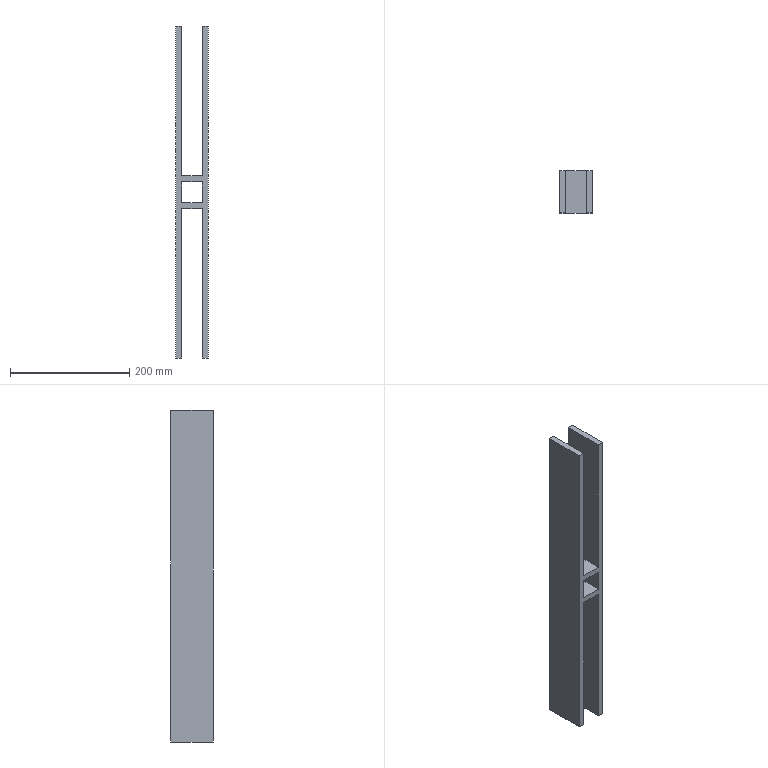Part | SolidWorks | features ICE 2, Extrusion 1 | 1 solid | 18 faces | box 55 x 71 x 556 mm | volume 839220 mm3 | plane 18
STEP:
#1=CARTESIAN_POINT('',(5.,-35.5,295.));
#2=VERTEX_POINT('',#1);
#3=CARTESIAN_POINT('',(5.,35.5,295.));
#4=VERTEX_POINT('',#3);
#5=CARTESIAN_POINT('',(5.,35.5,295.));
#6=DIRECTION('',(0.,1.,0.));
#7=VECTOR('',#6,1000.);
#8=LINE('',#5,#7);
#9=EDGE_CURVE('',#2,#4,#8,.T.);
#10=ORIENTED_EDGE('',*,*,#9,.F.);
#11=CARTESIAN_POINT('',(5.,-35.5,260.));
#12=VERTEX_POINT('',#11);
#13=CARTESIAN_POINT('',(5.,-35.5,556.));
#14=DIRECTION('',(0.,0.,-1.));
#15=VECTOR('',#14,1000.);
#16=LINE('',#13,#15);
#17=EDGE_CURVE('',#2,#12,#16,.T.);
#18=ORIENTED_EDGE('',*,*,#17,.T.);
#19=CARTESIAN_POINT('',(5.,35.5,260.));
#20=VERTEX_POINT('',#19);
#21=CARTESIAN_POINT('',(5.,35.5,260.));
#22=DIRECTION('',(0.,-1.,0.));
#23=VECTOR('',#22,1000.);
#24=LINE('',#21,#23);
#25=EDGE_CURVE('',#20,#12,#24,.T.);
#26=ORIENTED_EDGE('',*,*,#25,.F.);
#27=CARTESIAN_POINT('',(5.,35.5,556.));
#28=DIRECTION('',(0.,0.,-1.));
#29=VECTOR('',#28,1000.);
#30=LINE('',#27,#29);
#31=EDGE_CURVE('',#4,#20,#30,.T.);
#32=ORIENTED_EDGE('',*,*,#31,.F.);
#33=EDGE_LOOP('',(#10,#18,#26,#32));
#34=FACE_OUTER_BOUND('',#33,.T.);
#35=CARTESIAN_POINT('',(5.,35.5,556.));
#36=DIRECTION('',(-1.,0.,0.));
#37=DIRECTION('',(0.,-1.,0.));
#38=AXIS2_PLACEMENT_3D('',#35,#36,#37);
#39=PLANE('',#38);
#40=ADVANCED_FACE('',(#34),#39,.F.);
#41=CARTESIAN_POINT('',(5.,35.5,305.));
#42=VERTEX_POINT('',#41);
#43=CARTESIAN_POINT('',(5.,-35.5,305.));
#44=VERTEX_POINT('',#43);
#45=CARTESIAN_POINT('',(5.,35.5,305.));
#46=DIRECTION('',(0.,-1.,0.));
#47=VECTOR('',#46,1000.);
#48=LINE('',#45,#47);
#49=EDGE_CURVE('',#42,#44,#48,.T.);
#50=ORIENTED_EDGE('',*,*,#49,.F.);
#51=CARTESIAN_POINT('',(5.,35.5,556.));
#52=VERTEX_POINT('',#51);
#53=CARTESIAN_POINT('',(5.,35.5,556.));
#54=DIRECTION('',(0.,0.,-1.));
#55=VECTOR('',#54,1000.);
#56=LINE('',#53,#55);
#57=EDGE_CURVE('',#52,#42,#56,.T.);
#58=ORIENTED_EDGE('',*,*,#57,.F.);
#59=CARTESIAN_POINT('',(5.,-35.5,556.));
#60=VERTEX_POINT('',#59);
#61=CARTESIAN_POINT('',(5.,35.5,556.));
#62=DIRECTION('',(0.,1.,0.));
#63=VECTOR('',#62,1000.);
#64=LINE('',#61,#63);
#65=EDGE_CURVE('',#60,#52,#64,.T.);
#66=ORIENTED_EDGE('',*,*,#65,.F.);
#67=CARTESIAN_POINT('',(5.,-35.5,556.));
#68=DIRECTION('',(0.,0.,-1.));
#69=VECTOR('',#68,1000.);
#70=LINE('',#67,#69);
#71=EDGE_CURVE('',#60,#44,#70,.T.);
#72=ORIENTED_EDGE('',*,*,#71,.T.);
#73=EDGE_LOOP('',(#50,#58,#66,#72));
#74=FACE_OUTER_BOUND('',#73,.T.);
#75=CARTESIAN_POINT('',(5.,35.5,556.));
#76=DIRECTION('',(-1.,0.,0.));
#77=DIRECTION('',(0.,-1.,0.));
#78=AXIS2_PLACEMENT_3D('',#75,#76,#77);
#79=PLANE('',#78);
#80=ADVANCED_FACE('',(#74),#79,.F.);
#81=CARTESIAN_POINT('',(5.,-35.5,250.));
#82=VERTEX_POINT('',#81);
#83=CARTESIAN_POINT('',(5.,35.5,250.));
#84=VERTEX_POINT('',#83);
#85=CARTESIAN_POINT('',(5.,35.5,250.));
#86=DIRECTION('',(0.,1.,0.));
#87=VECTOR('',#86,1000.);
#88=LINE('',#85,#87);
#89=EDGE_CURVE('',#82,#84,#88,.T.);
#90=ORIENTED_EDGE('',*,*,#89,.F.);
#91=CARTESIAN_POINT('',(5.,-35.5,0.));
#92=VERTEX_POINT('',#91);
#93=CARTESIAN_POINT('',(5.,-35.5,556.));
#94=DIRECTION('',(0.,0.,-1.));
#95=VECTOR('',#94,1000.);
#96=LINE('',#93,#95);
#97=EDGE_CURVE('',#82,#92,#96,.T.);
#98=ORIENTED_EDGE('',*,*,#97,.T.);
#99=CARTESIAN_POINT('',(5.,35.5,0.));
#100=VERTEX_POINT('',#99);
#101=CARTESIAN_POINT('',(5.,35.5,0.));
#102=DIRECTION('',(0.,1.,0.));
#103=VECTOR('',#102,1000.);
#104=LINE('',#101,#103);
#105=EDGE_CURVE('',#92,#100,#104,.T.);
#106=ORIENTED_EDGE('',*,*,#105,.T.);
#107=CARTESIAN_POINT('',(5.,35.5,556.));
#108=DIRECTION('',(0.,0.,-1.));
#109=VECTOR('',#108,1000.);
#110=LINE('',#107,#109);
#111=EDGE_CURVE('',#84,#100,#110,.T.);
#112=ORIENTED_EDGE('',*,*,#111,.F.);
#113=EDGE_LOOP('',(#90,#98,#106,#112));
#114=FACE_OUTER_BOUND('',#113,.T.);
#115=CARTESIAN_POINT('',(5.,35.5,556.));
#116=DIRECTION('',(-1.,0.,0.));
#117=DIRECTION('',(0.,-1.,0.));
#118=AXIS2_PLACEMENT_3D('',#115,#116,#117);
#119=PLANE('',#118);
#120=ADVANCED_FACE('',(#114),#119,.F.);
#121=CARTESIAN_POINT('',(40.,35.5,260.));
#122=VERTEX_POINT('',#121);
#123=CARTESIAN_POINT('',(40.,35.5,260.));
#124=DIRECTION('',(-1.,0.,0.));
#125=VECTOR('',#124,1000.);
#126=LINE('',#123,#125);
#127=EDGE_CURVE('',#122,#20,#126,.T.);
#128=ORIENTED_EDGE('',*,*,#127,.F.);
#129=CARTESIAN_POINT('',(40.,35.5,295.));
#130=VERTEX_POINT('',#129);
#131=CARTESIAN_POINT('',(40.,35.5,556.));
#132=DIRECTION('',(0.,0.,1.));
#133=VECTOR('',#132,1000.);
#134=LINE('',#131,#133);
#135=EDGE_CURVE('',#122,#130,#134,.T.);
#136=ORIENTED_EDGE('',*,*,#135,.T.);
#137=CARTESIAN_POINT('',(40.,35.5,295.));
#138=DIRECTION('',(-1.,0.,0.));
#139=VECTOR('',#138,1000.);
#140=LINE('',#137,#139);
#141=EDGE_CURVE('',#130,#4,#140,.T.);
#142=ORIENTED_EDGE('',*,*,#141,.T.);
#143=ORIENTED_EDGE('',*,*,#31,.T.);
#144=EDGE_LOOP('',(#128,#136,#142,#143));
#145=FACE_BOUND('',#144,.T.);
#146=CARTESIAN_POINT('',(-5.,35.5,0.));
#147=VERTEX_POINT('',#146);
#148=CARTESIAN_POINT('',(-5.,35.5,0.));
#149=DIRECTION('',(-1.,0.,0.));
#150=VECTOR('',#149,1000.);
#151=LINE('',#148,#150);
#152=EDGE_CURVE('',#100,#147,#151,.T.);
#153=ORIENTED_EDGE('',*,*,#152,.T.);
#154=CARTESIAN_POINT('',(-5.,35.5,556.));
#155=VERTEX_POINT('',#154);
#156=CARTESIAN_POINT('',(-5.,35.5,556.));
#157=DIRECTION('',(0.,0.,-1.));
#158=VECTOR('',#157,1000.);
#159=LINE('',#156,#158);
#160=EDGE_CURVE('',#155,#147,#159,.T.);
#161=ORIENTED_EDGE('',*,*,#160,.F.);
#162=CARTESIAN_POINT('',(-5.,35.5,556.));
#163=DIRECTION('',(-1.,0.,0.));
#164=VECTOR('',#163,1000.);
#165=LINE('',#162,#164);
#166=EDGE_CURVE('',#52,#155,#165,.T.);
#167=ORIENTED_EDGE('',*,*,#166,.F.);
#168=ORIENTED_EDGE('',*,*,#57,.T.);
#169=CARTESIAN_POINT('',(40.,35.5,305.));
#170=VERTEX_POINT('',#169);
#171=CARTESIAN_POINT('',(40.,35.5,305.));
#172=DIRECTION('',(-1.,0.,0.));
#173=VECTOR('',#172,1000.);
#174=LINE('',#171,#173);
#175=EDGE_CURVE('',#170,#42,#174,.T.);
#176=ORIENTED_EDGE('',*,*,#175,.F.);
#177=CARTESIAN_POINT('',(40.,35.5,556.));
#178=VERTEX_POINT('',#177);
#179=CARTESIAN_POINT('',(40.,35.5,556.));
#180=DIRECTION('',(0.,0.,1.));
#181=VECTOR('',#180,1000.);
#182=LINE('',#179,#181);
#183=EDGE_CURVE('',#170,#178,#182,.T.);
#184=ORIENTED_EDGE('',*,*,#183,.T.);
#185=CARTESIAN_POINT('',(50.,35.5,556.));
#186=VERTEX_POINT('',#185);
#187=CARTESIAN_POINT('',(40.,35.5,556.));
#188=DIRECTION('',(1.,0.,0.));
#189=VECTOR('',#188,1000.);
#190=LINE('',#187,#189);
#191=EDGE_CURVE('',#178,#186,#190,.T.);
#192=ORIENTED_EDGE('',*,*,#191,.T.);
#193=CARTESIAN_POINT('',(50.,35.5,0.));
#194=VERTEX_POINT('',#193);
#195=CARTESIAN_POINT('',(50.,35.5,556.));
#196=DIRECTION('',(0.,0.,-1.));
#197=VECTOR('',#196,1000.);
#198=LINE('',#195,#197);
#199=EDGE_CURVE('',#186,#194,#198,.T.);
#200=ORIENTED_EDGE('',*,*,#199,.T.);
#201=CARTESIAN_POINT('',(40.,35.5,0.));
#202=VERTEX_POINT('',#201);
#203=CARTESIAN_POINT('',(40.,35.5,0.));
#204=DIRECTION('',(-1.,0.,0.));
#205=VECTOR('',#204,1000.);
#206=LINE('',#203,#205);
#207=EDGE_CURVE('',#194,#202,#206,.T.);
#208=ORIENTED_EDGE('',*,*,#207,.T.);
#209=CARTESIAN_POINT('',(40.,35.5,250.));
#210=VERTEX_POINT('',#209);
#211=CARTESIAN_POINT('',(40.,35.5,556.));
#212=DIRECTION('',(0.,0.,1.));
#213=VECTOR('',#212,1000.);
#214=LINE('',#211,#213);
#215=EDGE_CURVE('',#202,#210,#214,.T.);
#216=ORIENTED_EDGE('',*,*,#215,.T.);
#217=CARTESIAN_POINT('',(40.,35.5,250.));
#218=DIRECTION('',(-1.,0.,0.));
#219=VECTOR('',#218,1000.);
#220=LINE('',#217,#219);
#221=EDGE_CURVE('',#210,#84,#220,.T.);
#222=ORIENTED_EDGE('',*,*,#221,.T.);
#223=ORIENTED_EDGE('',*,*,#111,.T.);
#224=EDGE_LOOP('',(#153,#161,#167,#168,#176,#184,#192,#200,#208,#216,#222,#223));
#225=FACE_OUTER_BOUND('',#224,.T.);
#226=CARTESIAN_POINT('',(-5.,35.5,556.));
#227=DIRECTION('',(0.,-1.,0.));
#228=DIRECTION('',(0.,0.,-1.));
#229=AXIS2_PLACEMENT_3D('',#226,#227,#228);
#230=PLANE('',#229);
#231=ADVANCED_FACE('',(#145,#225),#230,.F.);
#232=CARTESIAN_POINT('',(-5.,-35.5,0.));
#233=VERTEX_POINT('',#232);
#234=CARTESIAN_POINT('',(-5.,35.5,0.));
#235=DIRECTION('',(0.,-1.,0.));
#236=VECTOR('',#235,1000.);
#237=LINE('',#234,#236);
#238=EDGE_CURVE('',#147,#233,#237,.T.);
#239=ORIENTED_EDGE('',*,*,#238,.T.);
#240=CARTESIAN_POINT('',(-5.,-35.5,556.));
#241=VERTEX_POINT('',#240);
#242=CARTESIAN_POINT('',(-5.,-35.5,556.));
#243=DIRECTION('',(0.,0.,-1.));
#244=VECTOR('',#243,1000.);
#245=LINE('',#242,#244);
#246=EDGE_CURVE('',#241,#233,#245,.T.);
#247=ORIENTED_EDGE('',*,*,#246,.F.);
#248=CARTESIAN_POINT('',(-5.,35.5,556.));
#249=DIRECTION('',(0.,-1.,0.));
#250=VECTOR('',#249,1000.);
#251=LINE('',#248,#250);
#252=EDGE_CURVE('',#155,#241,#251,.T.);
#253=ORIENTED_EDGE('',*,*,#252,.F.);
#254=ORIENTED_EDGE('',*,*,#160,.T.);
#255=EDGE_LOOP('',(#239,#247,#253,#254));
#256=FACE_OUTER_BOUND('',#255,.T.);
#257=CARTESIAN_POINT('',(-5.,35.5,556.));
#258=DIRECTION('',(1.,0.,0.));
#259=DIRECTION('',(0.,1.,0.));
#260=AXIS2_PLACEMENT_3D('',#257,#258,#259);
#261=PLANE('',#260);
#262=ADVANCED_FACE('',(#256),#261,.F.);
#263=CARTESIAN_POINT('',(40.,-35.5,250.));
#264=VERTEX_POINT('',#263);
#265=CARTESIAN_POINT('',(40.,-35.5,250.));
#266=DIRECTION('',(-1.,0.,0.));
#267=VECTOR('',#266,1000.);
#268=LINE('',#265,#267);
#269=EDGE_CURVE('',#264,#82,#268,.T.);
#270=ORIENTED_EDGE('',*,*,#269,.F.);
#271=CARTESIAN_POINT('',(40.,-35.5,0.));
#272=VERTEX_POINT('',#271);
#273=CARTESIAN_POINT('',(40.,-35.5,556.));
#274=DIRECTION('',(0.,0.,1.));
#275=VECTOR('',#274,1000.);
#276=LINE('',#273,#275);
#277=EDGE_CURVE('',#272,#264,#276,.T.);
#278=ORIENTED_EDGE('',*,*,#277,.F.);
#279=CARTESIAN_POINT('',(50.,-35.5,0.));
#280=VERTEX_POINT('',#279);
#281=CARTESIAN_POINT('',(40.,-35.5,0.));
#282=DIRECTION('',(-1.,0.,0.));
#283=VECTOR('',#282,1000.);
#284=LINE('',#281,#283);
#285=EDGE_CURVE('',#280,#272,#284,.T.);
#286=ORIENTED_EDGE('',*,*,#285,.F.);
#287=CARTESIAN_POINT('',(50.,-35.5,556.));
#288=VERTEX_POINT('',#287);
#289=CARTESIAN_POINT('',(50.,-35.5,556.));
#290=DIRECTION('',(0.,0.,-1.));
#291=VECTOR('',#290,1000.);
#292=LINE('',#289,#291);
#293=EDGE_CURVE('',#288,#280,#292,.T.);
#294=ORIENTED_EDGE('',*,*,#293,.F.);
#295=CARTESIAN_POINT('',(40.,-35.5,556.));
#296=VERTEX_POINT('',#295);
#297=CARTESIAN_POINT('',(40.,-35.5,556.));
#298=DIRECTION('',(1.,0.,0.));
#299=VECTOR('',#298,1000.);
#300=LINE('',#297,#299);
#301=EDGE_CURVE('',#296,#288,#300,.T.);
#302=ORIENTED_EDGE('',*,*,#301,.F.);
#303=CARTESIAN_POINT('',(40.,-35.5,305.));
#304=VERTEX_POINT('',#303);
#305=CARTESIAN_POINT('',(40.,-35.5,556.));
#306=DIRECTION('',(0.,0.,1.));
#307=VECTOR('',#306,1000.);
#308=LINE('',#305,#307);
#309=EDGE_CURVE('',#304,#296,#308,.T.);
#310=ORIENTED_EDGE('',*,*,#309,.F.);
#311=CARTESIAN_POINT('',(40.,-35.5,305.));
#312=DIRECTION('',(-1.,0.,0.));
#313=VECTOR('',#312,1000.);
#314=LINE('',#311,#313);
#315=EDGE_CURVE('',#304,#44,#314,.T.);
#316=ORIENTED_EDGE('',*,*,#315,.T.);
#317=ORIENTED_EDGE('',*,*,#71,.F.);
#318=CARTESIAN_POINT('',(-5.,-35.5,556.));
#319=DIRECTION('',(1.,0.,0.));
#320=VECTOR('',#319,1000.);
#321=LINE('',#318,#320);
#322=EDGE_CURVE('',#241,#60,#321,.T.);
#323=ORIENTED_EDGE('',*,*,#322,.F.);
#324=ORIENTED_EDGE('',*,*,#246,.T.);
#325=CARTESIAN_POINT('',(-5.,-35.5,0.));
#326=DIRECTION('',(1.,0.,0.));
#327=VECTOR('',#326,1000.);
#328=LINE('',#325,#327);
#329=EDGE_CURVE('',#233,#92,#328,.T.);
#330=ORIENTED_EDGE('',*,*,#329,.T.);
#331=ORIENTED_EDGE('',*,*,#97,.F.);
#332=EDGE_LOOP('',(#270,#278,#286,#294,#302,#310,#316,#317,#323,#324,#330,#331));
#333=FACE_OUTER_BOUND('',#332,.T.);
#334=CARTESIAN_POINT('',(40.,-35.5,260.));
#335=VERTEX_POINT('',#334);
#336=CARTESIAN_POINT('',(40.,-35.5,295.));
#337=VERTEX_POINT('',#336);
#338=CARTESIAN_POINT('',(40.,-35.5,556.));
#339=DIRECTION('',(0.,0.,1.));
#340=VECTOR('',#339,1000.);
#341=LINE('',#338,#340);
#342=EDGE_CURVE('',#335,#337,#341,.T.);
#343=ORIENTED_EDGE('',*,*,#342,.F.);
#344=CARTESIAN_POINT('',(40.,-35.5,260.));
#345=DIRECTION('',(-1.,0.,0.));
#346=VECTOR('',#345,1000.);
#347=LINE('',#344,#346);
#348=EDGE_CURVE('',#335,#12,#347,.T.);
#349=ORIENTED_EDGE('',*,*,#348,.T.);
#350=ORIENTED_EDGE('',*,*,#17,.F.);
#351=CARTESIAN_POINT('',(40.,-35.5,295.));
#352=DIRECTION('',(-1.,0.,0.));
#353=VECTOR('',#352,1000.);
#354=LINE('',#351,#353);
#355=EDGE_CURVE('',#337,#2,#354,.T.);
#356=ORIENTED_EDGE('',*,*,#355,.F.);
#357=EDGE_LOOP('',(#343,#349,#350,#356));
#358=FACE_BOUND('',#357,.T.);
#359=CARTESIAN_POINT('',(-5.,-35.5,556.));
#360=DIRECTION('',(0.,1.,0.));
#361=DIRECTION('',(0.,0.,1.));
#362=AXIS2_PLACEMENT_3D('',#359,#360,#361);
#363=PLANE('',#362);
#364=ADVANCED_FACE('',(#333,#358),#363,.F.);
#365=ORIENTED_EDGE('',*,*,#65,.T.);
#366=ORIENTED_EDGE('',*,*,#166,.T.);
#367=ORIENTED_EDGE('',*,*,#252,.T.);
#368=ORIENTED_EDGE('',*,*,#322,.T.);
#369=EDGE_LOOP('',(#365,#366,#367,#368));
#370=FACE_OUTER_BOUND('',#369,.T.);
#371=CARTESIAN_POINT('',(0.,0.,556.));
#372=DIRECTION('',(0.,0.,1.));
#373=DIRECTION('',(1.,0.,0.));
#374=AXIS2_PLACEMENT_3D('',#371,#372,#373);
#375=PLANE('',#374);
#376=ADVANCED_FACE('',(#370),#375,.T.);
#377=ORIENTED_EDGE('',*,*,#105,.F.);
#378=ORIENTED_EDGE('',*,*,#329,.F.);
#379=ORIENTED_EDGE('',*,*,#238,.F.);
#380=ORIENTED_EDGE('',*,*,#152,.F.);
#381=EDGE_LOOP('',(#377,#378,#379,#380));
#382=FACE_OUTER_BOUND('',#381,.T.);
#383=CARTESIAN_POINT('',(0.,0.,0.));
#384=DIRECTION('',(0.,0.,1.));
#385=DIRECTION('',(1.,0.,0.));
#386=AXIS2_PLACEMENT_3D('',#383,#384,#385);
#387=PLANE('',#386);
#388=ADVANCED_FACE('',(#382),#387,.F.);
#389=ORIENTED_EDGE('',*,*,#89,.T.);
#390=ORIENTED_EDGE('',*,*,#221,.F.);
#391=CARTESIAN_POINT('',(40.,35.5,250.));
#392=DIRECTION('',(0.,1.,0.));
#393=VECTOR('',#392,1000.);
#394=LINE('',#391,#393);
#395=EDGE_CURVE('',#264,#210,#394,.T.);
#396=ORIENTED_EDGE('',*,*,#395,.F.);
#397=ORIENTED_EDGE('',*,*,#269,.T.);
#398=EDGE_LOOP('',(#389,#390,#396,#397));
#399=FACE_OUTER_BOUND('',#398,.T.);
#400=CARTESIAN_POINT('',(40.,35.5,250.));
#401=DIRECTION('',(0.,0.,1.));
#402=DIRECTION('',(1.,0.,0.));
#403=AXIS2_PLACEMENT_3D('',#400,#401,#402);
#404=PLANE('',#403);
#405=ADVANCED_FACE('',(#399),#404,.F.);
#406=ORIENTED_EDGE('',*,*,#25,.T.);
#407=ORIENTED_EDGE('',*,*,#348,.F.);
#408=CARTESIAN_POINT('',(40.,35.5,260.));
#409=DIRECTION('',(0.,-1.,0.));
#410=VECTOR('',#409,1000.);
#411=LINE('',#408,#410);
#412=EDGE_CURVE('',#122,#335,#411,.T.);
#413=ORIENTED_EDGE('',*,*,#412,.F.);
#414=ORIENTED_EDGE('',*,*,#127,.T.);
#415=EDGE_LOOP('',(#406,#407,#413,#414));
#416=FACE_OUTER_BOUND('',#415,.T.);
#417=CARTESIAN_POINT('',(40.,35.5,260.));
#418=DIRECTION('',(0.,0.,-1.));
#419=DIRECTION('',(-1.,0.,0.));
#420=AXIS2_PLACEMENT_3D('',#417,#418,#419);
#421=PLANE('',#420);
#422=ADVANCED_FACE('',(#416),#421,.F.);
#423=ORIENTED_EDGE('',*,*,#9,.T.);
#424=ORIENTED_EDGE('',*,*,#141,.F.);
#425=CARTESIAN_POINT('',(40.,35.5,295.));
#426=DIRECTION('',(0.,1.,0.));
#427=VECTOR('',#426,1000.);
#428=LINE('',#425,#427);
#429=EDGE_CURVE('',#337,#130,#428,.T.);
#430=ORIENTED_EDGE('',*,*,#429,.F.);
#431=ORIENTED_EDGE('',*,*,#355,.T.);
#432=EDGE_LOOP('',(#423,#424,#430,#431));
#433=FACE_OUTER_BOUND('',#432,.T.);
#434=CARTESIAN_POINT('',(40.,35.5,295.));
#435=DIRECTION('',(0.,0.,1.));
#436=DIRECTION('',(1.,0.,0.));
#437=AXIS2_PLACEMENT_3D('',#434,#435,#436);
#438=PLANE('',#437);
#439=ADVANCED_FACE('',(#433),#438,.F.);
#440=ORIENTED_EDGE('',*,*,#49,.T.);
#441=ORIENTED_EDGE('',*,*,#315,.F.);
#442=CARTESIAN_POINT('',(40.,35.5,305.));
#443=DIRECTION('',(0.,-1.,0.));
#444=VECTOR('',#443,1000.);
#445=LINE('',#442,#444);
#446=EDGE_CURVE('',#170,#304,#445,.T.);
#447=ORIENTED_EDGE('',*,*,#446,.F.);
#448=ORIENTED_EDGE('',*,*,#175,.T.);
#449=EDGE_LOOP('',(#440,#441,#447,#448));
#450=FACE_OUTER_BOUND('',#449,.T.);
#451=CARTESIAN_POINT('',(40.,35.5,305.));
#452=DIRECTION('',(0.,0.,-1.));
#453=DIRECTION('',(-1.,0.,0.));
#454=AXIS2_PLACEMENT_3D('',#451,#452,#453);
#455=PLANE('',#454);
#456=ADVANCED_FACE('',(#450),#455,.F.);
#457=ORIENTED_EDGE('',*,*,#395,.T.);
#458=ORIENTED_EDGE('',*,*,#215,.F.);
#459=CARTESIAN_POINT('',(40.,-35.5,0.));
#460=DIRECTION('',(0.,1.,0.));
#461=VECTOR('',#460,1000.);
#462=LINE('',#459,#461);
#463=EDGE_CURVE('',#272,#202,#462,.T.);
#464=ORIENTED_EDGE('',*,*,#463,.F.);
#465=ORIENTED_EDGE('',*,*,#277,.T.);
#466=EDGE_LOOP('',(#457,#458,#464,#465));
#467=FACE_OUTER_BOUND('',#466,.T.);
#468=CARTESIAN_POINT('',(40.,-35.5,556.));
#469=DIRECTION('',(-1.,0.,0.));
#470=DIRECTION('',(0.,0.,1.));
#471=AXIS2_PLACEMENT_3D('',#468,#469,#470);
#472=PLANE('',#471);
#473=ADVANCED_FACE('',(#467),#472,.T.);
#474=ORIENTED_EDGE('',*,*,#412,.T.);
#475=ORIENTED_EDGE('',*,*,#342,.T.);
#476=ORIENTED_EDGE('',*,*,#429,.T.);
#477=ORIENTED_EDGE('',*,*,#135,.F.);
#478=EDGE_LOOP('',(#474,#475,#476,#477));
#479=FACE_OUTER_BOUND('',#478,.T.);
#480=CARTESIAN_POINT('',(40.,-35.5,556.));
#481=DIRECTION('',(-1.,0.,0.));
#482=DIRECTION('',(0.,0.,1.));
#483=AXIS2_PLACEMENT_3D('',#480,#481,#482);
#484=PLANE('',#483);
#485=ADVANCED_FACE('',(#479),#484,.T.);
#486=ORIENTED_EDGE('',*,*,#446,.T.);
#487=ORIENTED_EDGE('',*,*,#309,.T.);
#488=CARTESIAN_POINT('',(40.,-35.5,556.));
#489=DIRECTION('',(0.,1.,0.));
#490=VECTOR('',#489,1000.);
#491=LINE('',#488,#490);
#492=EDGE_CURVE('',#296,#178,#491,.T.);
#493=ORIENTED_EDGE('',*,*,#492,.T.);
#494=ORIENTED_EDGE('',*,*,#183,.F.);
#495=EDGE_LOOP('',(#486,#487,#493,#494));
#496=FACE_OUTER_BOUND('',#495,.T.);
#497=CARTESIAN_POINT('',(40.,-35.5,556.));
#498=DIRECTION('',(-1.,0.,0.));
#499=DIRECTION('',(0.,0.,1.));
#500=AXIS2_PLACEMENT_3D('',#497,#498,#499);
#501=PLANE('',#500);
#502=ADVANCED_FACE('',(#496),#501,.T.);
#503=ORIENTED_EDGE('',*,*,#207,.F.);
#504=CARTESIAN_POINT('',(50.,-35.5,0.));
#505=DIRECTION('',(0.,1.,0.));
#506=VECTOR('',#505,1000.);
#507=LINE('',#504,#506);
#508=EDGE_CURVE('',#280,#194,#507,.T.);
#509=ORIENTED_EDGE('',*,*,#508,.F.);
#510=ORIENTED_EDGE('',*,*,#285,.T.);
#511=ORIENTED_EDGE('',*,*,#463,.T.);
#512=EDGE_LOOP('',(#503,#509,#510,#511));
#513=FACE_OUTER_BOUND('',#512,.T.);
#514=CARTESIAN_POINT('',(40.,-35.5,0.));
#515=DIRECTION('',(0.,0.,-1.));
#516=DIRECTION('',(-1.,0.,0.));
#517=AXIS2_PLACEMENT_3D('',#514,#515,#516);
#518=PLANE('',#517);
#519=ADVANCED_FACE('',(#513),#518,.T.);
#520=ORIENTED_EDGE('',*,*,#199,.F.);
#521=CARTESIAN_POINT('',(50.,-35.5,556.));
#522=DIRECTION('',(0.,1.,0.));
#523=VECTOR('',#522,1000.);
#524=LINE('',#521,#523);
#525=EDGE_CURVE('',#288,#186,#524,.T.);
#526=ORIENTED_EDGE('',*,*,#525,.F.);
#527=ORIENTED_EDGE('',*,*,#293,.T.);
#528=ORIENTED_EDGE('',*,*,#508,.T.);
#529=EDGE_LOOP('',(#520,#526,#527,#528));
#530=FACE_OUTER_BOUND('',#529,.T.);
#531=CARTESIAN_POINT('',(50.,-35.5,556.));
#532=DIRECTION('',(1.,0.,0.));
#533=DIRECTION('',(0.,0.,-1.));
#534=AXIS2_PLACEMENT_3D('',#531,#532,#533);
#535=PLANE('',#534);
#536=ADVANCED_FACE('',(#530),#535,.T.);
#537=ORIENTED_EDGE('',*,*,#191,.F.);
#538=ORIENTED_EDGE('',*,*,#492,.F.);
#539=ORIENTED_EDGE('',*,*,#301,.T.);
#540=ORIENTED_EDGE('',*,*,#525,.T.);
#541=EDGE_LOOP('',(#537,#538,#539,#540));
#542=FACE_OUTER_BOUND('',#541,.T.);
#543=CARTESIAN_POINT('',(40.,-35.5,556.));
#544=DIRECTION('',(0.,0.,1.));
#545=DIRECTION('',(1.,0.,0.));
#546=AXIS2_PLACEMENT_3D('',#543,#544,#545);
#547=PLANE('',#546);
#548=ADVANCED_FACE('',(#542),#547,.T.);
#549=CLOSED_SHELL('',(#40,#80,#120,#231,#262,#364,#376,#388,#405,#422,#439,#456,#473,#485,#502,#519,#536,#548));
#550=MANIFOLD_SOLID_BREP('',#549);
#551=CARTESIAN_POINT('',(0.,0.,0.));
#552=DIRECTION('',(0.,0.,1.));
#553=DIRECTION('',(1.,0.,0.));
#554=AXIS2_PLACEMENT_3D('',#551,#552,#553);
#555=(LENGTH_UNIT()NAMED_UNIT(*)SI_UNIT(.MILLI.,.METRE.));
#556=UNCERTAINTY_MEASURE_WITH_UNIT(LENGTH_MEASURE(0.00001),#555,'','');
#557=(NAMED_UNIT(*)PLANE_ANGLE_UNIT()SI_UNIT($,.RADIAN.));
#558=(NAMED_UNIT(*)SI_UNIT($,.STERADIAN.)SOLID_ANGLE_UNIT());
#559=(GEOMETRIC_REPRESENTATION_CONTEXT(3)GLOBAL_UNCERTAINTY_ASSIGNED_CONTEXT((#556))GLOBAL_UNIT_ASSIGNED_CONTEXT((#555,#557,#558))REPRESENTATION_CONTEXT('',''));
#560=ADVANCED_BREP_SHAPE_REPRESENTATION('',(#550,#554),#559);